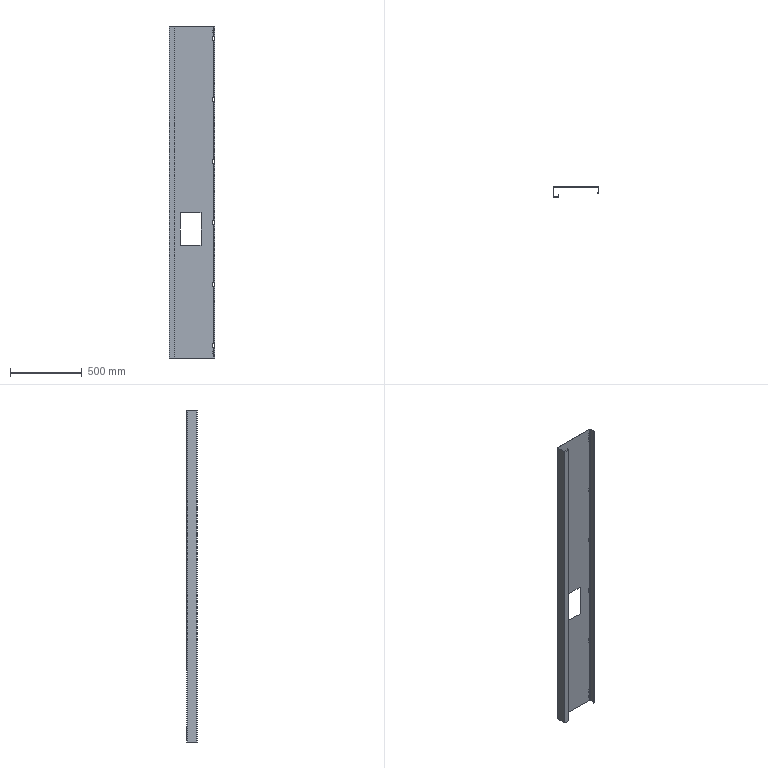Part | 1 solid | 148 faces | box 320 x 70 x 2316 mm | volume 1322236 mm3 | plane 84 | cylinder 64 | commonest cylinder face diameters 6.2 x28 9 x18 4 x8 1 x5 3.4 x5